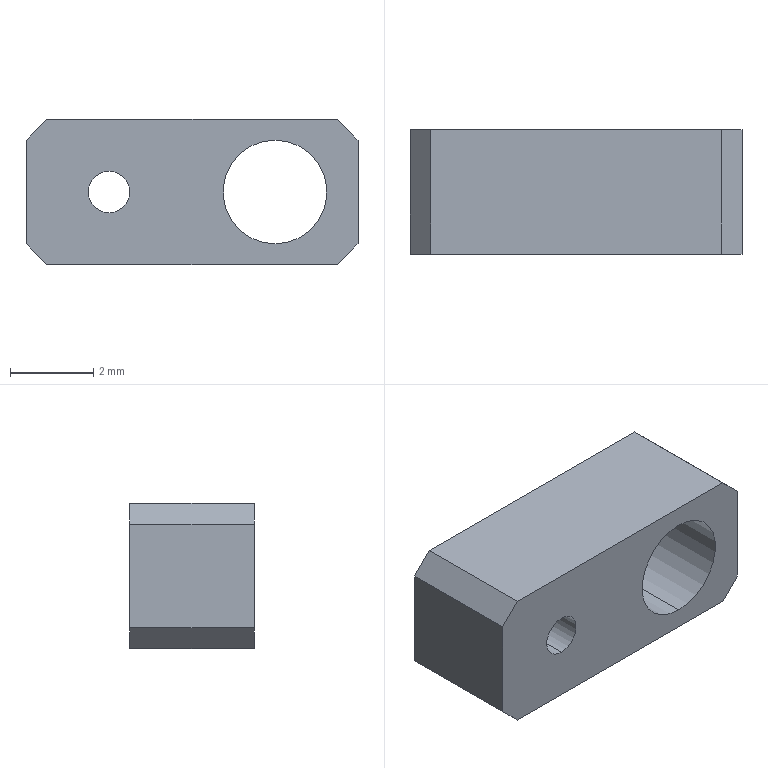Part | SolidWorks | features HoleWzd 2, Chamfer 1, Extrusion 1, ICE 1 | 1 solid | 17 faces | box 8 x 3 x 3.5 mm | volume 57.171 mm3 | plane 11 | cylinder 6 | commonest cylinder face diameters 2.5 x4 1 x2
STEP:
#1=CARTESIAN_POINT('',(2.,1.5,1.25));
#2=VERTEX_POINT('',#1);
#3=CARTESIAN_POINT('',(2.,1.5,-1.25));
#4=VERTEX_POINT('',#3);
#5=CARTESIAN_POINT('',(2.,1.5,0.));
#6=DIRECTION('',(0.,-1.,0.));
#7=DIRECTION('',(0.,0.,-1.));
#8=AXIS2_PLACEMENT_3D('',#5,#6,#7);
#9=CIRCLE('',#8,1.25);
#10=EDGE_CURVE('',#2,#4,#9,.T.);
#11=ORIENTED_EDGE('',*,*,#10,.F.);
#12=CARTESIAN_POINT('',(2.,-1.5,1.25));
#13=VERTEX_POINT('',#12);
#14=CARTESIAN_POINT('',(2.,-1.5,1.25));
#15=DIRECTION('',(0.,-1.,0.));
#16=VECTOR('',#15,1000.);
#17=LINE('',#14,#16);
#18=EDGE_CURVE('',#2,#13,#17,.T.);
#19=ORIENTED_EDGE('',*,*,#18,.T.);
#20=CARTESIAN_POINT('',(2.,-1.5,-1.25));
#21=VERTEX_POINT('',#20);
#22=CARTESIAN_POINT('',(2.,-1.5,0.));
#23=DIRECTION('',(0.,-1.,0.));
#24=DIRECTION('',(0.,0.,-1.));
#25=AXIS2_PLACEMENT_3D('',#22,#23,#24);
#26=CIRCLE('',#25,1.25);
#27=EDGE_CURVE('',#13,#21,#26,.T.);
#28=ORIENTED_EDGE('',*,*,#27,.T.);
#29=CARTESIAN_POINT('',(2.,-1.5,-1.25));
#30=DIRECTION('',(0.,-1.,0.));
#31=VECTOR('',#30,1000.);
#32=LINE('',#29,#31);
#33=EDGE_CURVE('',#4,#21,#32,.T.);
#34=ORIENTED_EDGE('',*,*,#33,.F.);
#35=EDGE_LOOP('',(#11,#19,#28,#34));
#36=FACE_OUTER_BOUND('',#35,.T.);
#37=CARTESIAN_POINT('',(2.,-1.5,0.));
#38=DIRECTION('',(0.,-1.,0.));
#39=DIRECTION('',(0.,0.,-1.));
#40=AXIS2_PLACEMENT_3D('',#37,#38,#39);
#41=CYLINDRICAL_SURFACE('',#40,1.25);
#42=ADVANCED_FACE('',(#36),#41,.F.);
#43=CARTESIAN_POINT('',(-2.,-0.5,-0.5));
#44=VERTEX_POINT('',#43);
#45=CARTESIAN_POINT('',(-2.,-0.5,0.5));
#46=VERTEX_POINT('',#45);
#47=CARTESIAN_POINT('',(-2.,-0.5,0.));
#48=DIRECTION('',(0.,1.,0.));
#49=DIRECTION('',(0.,0.,1.));
#50=AXIS2_PLACEMENT_3D('',#47,#48,#49);
#51=CIRCLE('',#50,0.5);
#52=EDGE_CURVE('',#44,#46,#51,.T.);
#53=ORIENTED_EDGE('',*,*,#52,.T.);
#54=CARTESIAN_POINT('',(-2.,-1.5,0.5));
#55=VERTEX_POINT('',#54);
#56=CARTESIAN_POINT('',(-2.,-1.5,0.5));
#57=DIRECTION('',(0.,-1.,0.));
#58=VECTOR('',#57,1000.);
#59=LINE('',#56,#58);
#60=EDGE_CURVE('',#46,#55,#59,.T.);
#61=ORIENTED_EDGE('',*,*,#60,.T.);
#62=CARTESIAN_POINT('',(-2.,-1.5,-0.5));
#63=VERTEX_POINT('',#62);
#64=CARTESIAN_POINT('',(-2.,-1.5,0.));
#65=DIRECTION('',(0.,-1.,0.));
#66=DIRECTION('',(0.,0.,-1.));
#67=AXIS2_PLACEMENT_3D('',#64,#65,#66);
#68=CIRCLE('',#67,0.5);
#69=EDGE_CURVE('',#55,#63,#68,.T.);
#70=ORIENTED_EDGE('',*,*,#69,.T.);
#71=CARTESIAN_POINT('',(-2.,-1.5,-0.5));
#72=DIRECTION('',(0.,-1.,0.));
#73=VECTOR('',#72,1000.);
#74=LINE('',#71,#73);
#75=EDGE_CURVE('',#44,#63,#74,.T.);
#76=ORIENTED_EDGE('',*,*,#75,.F.);
#77=EDGE_LOOP('',(#53,#61,#70,#76));
#78=FACE_OUTER_BOUND('',#77,.T.);
#79=CARTESIAN_POINT('',(-2.,-1.5,0.));
#80=DIRECTION('',(0.,-1.,0.));
#81=DIRECTION('',(0.,0.,-1.));
#82=AXIS2_PLACEMENT_3D('',#79,#80,#81);
#83=CYLINDRICAL_SURFACE('',#82,0.5);
#84=ADVANCED_FACE('',(#78),#83,.F.);
#85=CARTESIAN_POINT('',(-2.,-0.5,-1.25));
#86=VERTEX_POINT('',#85);
#87=CARTESIAN_POINT('',(-2.,-0.5,1.25));
#88=VERTEX_POINT('',#87);
#89=CARTESIAN_POINT('',(-2.,-0.5,0.));
#90=DIRECTION('',(0.,1.,0.));
#91=DIRECTION('',(0.,0.,1.));
#92=AXIS2_PLACEMENT_3D('',#89,#90,#91);
#93=CIRCLE('',#92,1.25);
#94=EDGE_CURVE('',#86,#88,#93,.T.);
#95=ORIENTED_EDGE('',*,*,#94,.F.);
#96=CARTESIAN_POINT('',(-2.,1.5,-1.25));
#97=VERTEX_POINT('',#96);
#98=CARTESIAN_POINT('',(-2.,-0.5,-1.25));
#99=DIRECTION('',(0.,1.,0.));
#100=VECTOR('',#99,1000.);
#101=LINE('',#98,#100);
#102=EDGE_CURVE('',#86,#97,#101,.T.);
#103=ORIENTED_EDGE('',*,*,#102,.T.);
#104=CARTESIAN_POINT('',(-2.,1.5,1.25));
#105=VERTEX_POINT('',#104);
#106=CARTESIAN_POINT('',(-2.,1.5,0.));
#107=DIRECTION('',(0.,1.,0.));
#108=DIRECTION('',(0.,0.,1.));
#109=AXIS2_PLACEMENT_3D('',#106,#107,#108);
#110=CIRCLE('',#109,1.25);
#111=EDGE_CURVE('',#97,#105,#110,.T.);
#112=ORIENTED_EDGE('',*,*,#111,.T.);
#113=CARTESIAN_POINT('',(-2.,-0.5,1.25));
#114=DIRECTION('',(0.,1.,0.));
#115=VECTOR('',#114,1000.);
#116=LINE('',#113,#115);
#117=EDGE_CURVE('',#88,#105,#116,.T.);
#118=ORIENTED_EDGE('',*,*,#117,.F.);
#119=EDGE_LOOP('',(#95,#103,#112,#118));
#120=FACE_OUTER_BOUND('',#119,.T.);
#121=CARTESIAN_POINT('',(-2.,-0.5,0.));
#122=DIRECTION('',(0.,1.,0.));
#123=DIRECTION('',(0.,0.,1.));
#124=AXIS2_PLACEMENT_3D('',#121,#122,#123);
#125=CYLINDRICAL_SURFACE('',#124,1.25);
#126=ADVANCED_FACE('',(#120),#125,.F.);
#127=CARTESIAN_POINT('',(4.,1.5,1.25));
#128=VERTEX_POINT('',#127);
#129=CARTESIAN_POINT('',(4.,1.5,-1.25));
#130=VERTEX_POINT('',#129);
#131=CARTESIAN_POINT('',(4.,1.5,-1.75));
#132=DIRECTION('',(0.,0.,-1.));
#133=VECTOR('',#132,1000.);
#134=LINE('',#131,#133);
#135=EDGE_CURVE('',#128,#130,#134,.T.);
#136=ORIENTED_EDGE('',*,*,#135,.F.);
#137=CARTESIAN_POINT('',(4.,-1.5,1.25));
#138=VERTEX_POINT('',#137);
#139=CARTESIAN_POINT('',(4.,1.5,1.25));
#140=DIRECTION('',(0.,-1.,0.));
#141=VECTOR('',#140,1000.);
#142=LINE('',#139,#141);
#143=EDGE_CURVE('',#128,#138,#142,.T.);
#144=ORIENTED_EDGE('',*,*,#143,.T.);
#145=CARTESIAN_POINT('',(4.,-1.5,-1.25));
#146=VERTEX_POINT('',#145);
#147=CARTESIAN_POINT('',(4.,-1.5,-1.75));
#148=DIRECTION('',(0.,0.,-1.));
#149=VECTOR('',#148,1000.);
#150=LINE('',#147,#149);
#151=EDGE_CURVE('',#138,#146,#150,.T.);
#152=ORIENTED_EDGE('',*,*,#151,.T.);
#153=CARTESIAN_POINT('',(4.,1.5,-1.25));
#154=DIRECTION('',(0.,1.,0.));
#155=VECTOR('',#154,1000.);
#156=LINE('',#153,#155);
#157=EDGE_CURVE('',#146,#130,#156,.T.);
#158=ORIENTED_EDGE('',*,*,#157,.T.);
#159=EDGE_LOOP('',(#136,#144,#152,#158));
#160=FACE_OUTER_BOUND('',#159,.T.);
#161=CARTESIAN_POINT('',(4.,1.5,-1.75));
#162=DIRECTION('',(-1.,0.,0.));
#163=DIRECTION('',(0.,0.,1.));
#164=AXIS2_PLACEMENT_3D('',#161,#162,#163);
#165=PLANE('',#164);
#166=ADVANCED_FACE('',(#160),#165,.F.);
#167=CARTESIAN_POINT('',(3.5,1.5,-1.75));
#168=VERTEX_POINT('',#167);
#169=CARTESIAN_POINT('',(-3.5,1.5,-1.75));
#170=VERTEX_POINT('',#169);
#171=CARTESIAN_POINT('',(-4.,1.5,-1.75));
#172=DIRECTION('',(-1.,0.,0.));
#173=VECTOR('',#172,1000.);
#174=LINE('',#171,#173);
#175=EDGE_CURVE('',#168,#170,#174,.T.);
#176=ORIENTED_EDGE('',*,*,#175,.F.);
#177=CARTESIAN_POINT('',(3.5,-1.5,-1.75));
#178=VERTEX_POINT('',#177);
#179=CARTESIAN_POINT('',(3.5,1.5,-1.75));
#180=DIRECTION('',(0.,-1.,0.));
#181=VECTOR('',#180,1000.);
#182=LINE('',#179,#181);
#183=EDGE_CURVE('',#168,#178,#182,.T.);
#184=ORIENTED_EDGE('',*,*,#183,.T.);
#185=CARTESIAN_POINT('',(-3.5,-1.5,-1.75));
#186=VERTEX_POINT('',#185);
#187=CARTESIAN_POINT('',(-4.,-1.5,-1.75));
#188=DIRECTION('',(-1.,0.,0.));
#189=VECTOR('',#188,1000.);
#190=LINE('',#187,#189);
#191=EDGE_CURVE('',#178,#186,#190,.T.);
#192=ORIENTED_EDGE('',*,*,#191,.T.);
#193=CARTESIAN_POINT('',(-3.5,1.5,-1.75));
#194=DIRECTION('',(0.,1.,0.));
#195=VECTOR('',#194,1000.);
#196=LINE('',#193,#195);
#197=EDGE_CURVE('',#186,#170,#196,.T.);
#198=ORIENTED_EDGE('',*,*,#197,.T.);
#199=EDGE_LOOP('',(#176,#184,#192,#198));
#200=FACE_OUTER_BOUND('',#199,.T.);
#201=CARTESIAN_POINT('',(-4.,1.5,-1.75));
#202=DIRECTION('',(0.,0.,1.));
#203=DIRECTION('',(1.,0.,0.));
#204=AXIS2_PLACEMENT_3D('',#201,#202,#203);
#205=PLANE('',#204);
#206=ADVANCED_FACE('',(#200),#205,.F.);
#207=CARTESIAN_POINT('',(-4.,-1.5,-1.25));
#208=VERTEX_POINT('',#207);
#209=CARTESIAN_POINT('',(-4.,-1.5,1.25));
#210=VERTEX_POINT('',#209);
#211=CARTESIAN_POINT('',(-4.,-1.5,-1.75));
#212=DIRECTION('',(0.,0.,1.));
#213=VECTOR('',#212,1000.);
#214=LINE('',#211,#213);
#215=EDGE_CURVE('',#208,#210,#214,.T.);
#216=ORIENTED_EDGE('',*,*,#215,.T.);
#217=CARTESIAN_POINT('',(-4.,1.5,1.25));
#218=VERTEX_POINT('',#217);
#219=CARTESIAN_POINT('',(-4.,1.5,1.25));
#220=DIRECTION('',(0.,1.,0.));
#221=VECTOR('',#220,1000.);
#222=LINE('',#219,#221);
#223=EDGE_CURVE('',#210,#218,#222,.T.);
#224=ORIENTED_EDGE('',*,*,#223,.T.);
#225=CARTESIAN_POINT('',(-4.,1.5,-1.25));
#226=VERTEX_POINT('',#225);
#227=CARTESIAN_POINT('',(-4.,1.5,-1.75));
#228=DIRECTION('',(0.,0.,1.));
#229=VECTOR('',#228,1000.);
#230=LINE('',#227,#229);
#231=EDGE_CURVE('',#226,#218,#230,.T.);
#232=ORIENTED_EDGE('',*,*,#231,.F.);
#233=CARTESIAN_POINT('',(-4.,1.5,-1.25));
#234=DIRECTION('',(0.,-1.,0.));
#235=VECTOR('',#234,1000.);
#236=LINE('',#233,#235);
#237=EDGE_CURVE('',#226,#208,#236,.T.);
#238=ORIENTED_EDGE('',*,*,#237,.T.);
#239=EDGE_LOOP('',(#216,#224,#232,#238));
#240=FACE_OUTER_BOUND('',#239,.T.);
#241=CARTESIAN_POINT('',(-4.,1.5,-1.75));
#242=DIRECTION('',(1.,0.,0.));
#243=DIRECTION('',(0.,0.,-1.));
#244=AXIS2_PLACEMENT_3D('',#241,#242,#243);
#245=PLANE('',#244);
#246=ADVANCED_FACE('',(#240),#245,.F.);
#247=CARTESIAN_POINT('',(-3.5,-1.5,1.75));
#248=VERTEX_POINT('',#247);
#249=CARTESIAN_POINT('',(3.5,-1.5,1.75));
#250=VERTEX_POINT('',#249);
#251=CARTESIAN_POINT('',(-4.,-1.5,1.75));
#252=DIRECTION('',(1.,0.,0.));
#253=VECTOR('',#252,1000.);
#254=LINE('',#251,#253);
#255=EDGE_CURVE('',#248,#250,#254,.T.);
#256=ORIENTED_EDGE('',*,*,#255,.T.);
#257=CARTESIAN_POINT('',(3.5,1.5,1.75));
#258=VERTEX_POINT('',#257);
#259=CARTESIAN_POINT('',(3.5,1.5,1.75));
#260=DIRECTION('',(0.,1.,0.));
#261=VECTOR('',#260,1000.);
#262=LINE('',#259,#261);
#263=EDGE_CURVE('',#250,#258,#262,.T.);
#264=ORIENTED_EDGE('',*,*,#263,.T.);
#265=CARTESIAN_POINT('',(-3.5,1.5,1.75));
#266=VERTEX_POINT('',#265);
#267=CARTESIAN_POINT('',(-4.,1.5,1.75));
#268=DIRECTION('',(1.,0.,0.));
#269=VECTOR('',#268,1000.);
#270=LINE('',#267,#269);
#271=EDGE_CURVE('',#266,#258,#270,.T.);
#272=ORIENTED_EDGE('',*,*,#271,.F.);
#273=CARTESIAN_POINT('',(-3.5,1.5,1.75));
#274=DIRECTION('',(0.,-1.,0.));
#275=VECTOR('',#274,1000.);
#276=LINE('',#273,#275);
#277=EDGE_CURVE('',#266,#248,#276,.T.);
#278=ORIENTED_EDGE('',*,*,#277,.T.);
#279=EDGE_LOOP('',(#256,#264,#272,#278));
#280=FACE_OUTER_BOUND('',#279,.T.);
#281=CARTESIAN_POINT('',(-4.,1.5,1.75));
#282=DIRECTION('',(0.,0.,-1.));
#283=DIRECTION('',(-1.,0.,0.));
#284=AXIS2_PLACEMENT_3D('',#281,#282,#283);
#285=PLANE('',#284);
#286=ADVANCED_FACE('',(#280),#285,.F.);
#287=CARTESIAN_POINT('',(2.,1.5,0.));
#288=DIRECTION('',(0.,-1.,0.));
#289=DIRECTION('',(0.,0.,-1.));
#290=AXIS2_PLACEMENT_3D('',#287,#288,#289);
#291=CIRCLE('',#290,1.25);
#292=EDGE_CURVE('',#4,#2,#291,.T.);
#293=ORIENTED_EDGE('',*,*,#292,.T.);
#294=ORIENTED_EDGE('',*,*,#10,.T.);
#295=EDGE_LOOP('',(#293,#294));
#296=FACE_BOUND('',#295,.T.);
#297=CARTESIAN_POINT('',(-2.,1.5,0.));
#298=DIRECTION('',(0.,1.,0.));
#299=DIRECTION('',(0.,0.,1.));
#300=AXIS2_PLACEMENT_3D('',#297,#298,#299);
#301=CIRCLE('',#300,1.25);
#302=EDGE_CURVE('',#105,#97,#301,.T.);
#303=ORIENTED_EDGE('',*,*,#302,.F.);
#304=ORIENTED_EDGE('',*,*,#111,.F.);
#305=EDGE_LOOP('',(#303,#304));
#306=FACE_BOUND('',#305,.T.);
#307=ORIENTED_EDGE('',*,*,#271,.T.);
#308=CARTESIAN_POINT('',(2.625,1.5,2.625));
#309=DIRECTION('',(0.7071,0.,-0.7071));
#310=VECTOR('',#309,1000.);
#311=LINE('',#308,#310);
#312=EDGE_CURVE('',#258,#128,#311,.T.);
#313=ORIENTED_EDGE('',*,*,#312,.T.);
#314=ORIENTED_EDGE('',*,*,#135,.T.);
#315=CARTESIAN_POINT('',(2.625,1.5,-2.625));
#316=DIRECTION('',(-0.7071,0.,-0.7071));
#317=VECTOR('',#316,1000.);
#318=LINE('',#315,#317);
#319=EDGE_CURVE('',#130,#168,#318,.T.);
#320=ORIENTED_EDGE('',*,*,#319,.T.);
#321=ORIENTED_EDGE('',*,*,#175,.T.);
#322=CARTESIAN_POINT('',(-2.625,1.5,-2.625));
#323=DIRECTION('',(-0.7071,0.,0.7071));
#324=VECTOR('',#323,1000.);
#325=LINE('',#322,#324);
#326=EDGE_CURVE('',#170,#226,#325,.T.);
#327=ORIENTED_EDGE('',*,*,#326,.T.);
#328=ORIENTED_EDGE('',*,*,#231,.T.);
#329=CARTESIAN_POINT('',(-2.625,1.5,2.625));
#330=DIRECTION('',(0.7071,0.,0.7071));
#331=VECTOR('',#330,1000.);
#332=LINE('',#329,#331);
#333=EDGE_CURVE('',#218,#266,#332,.T.);
#334=ORIENTED_EDGE('',*,*,#333,.T.);
#335=EDGE_LOOP('',(#307,#313,#314,#320,#321,#327,#328,#334));
#336=FACE_OUTER_BOUND('',#335,.T.);
#337=CARTESIAN_POINT('',(0.,1.5,0.));
#338=DIRECTION('',(0.,1.,0.));
#339=DIRECTION('',(0.,0.,1.));
#340=AXIS2_PLACEMENT_3D('',#337,#338,#339);
#341=PLANE('',#340);
#342=ADVANCED_FACE('',(#296,#306,#336),#341,.T.);
#343=CARTESIAN_POINT('',(2.,-1.5,0.));
#344=DIRECTION('',(0.,-1.,0.));
#345=DIRECTION('',(0.,0.,-1.));
#346=AXIS2_PLACEMENT_3D('',#343,#344,#345);
#347=CIRCLE('',#346,1.25);
#348=EDGE_CURVE('',#21,#13,#347,.T.);
#349=ORIENTED_EDGE('',*,*,#348,.F.);
#350=ORIENTED_EDGE('',*,*,#27,.F.);
#351=EDGE_LOOP('',(#349,#350));
#352=FACE_BOUND('',#351,.T.);
#353=CARTESIAN_POINT('',(-2.,-1.5,0.));
#354=DIRECTION('',(0.,-1.,0.));
#355=DIRECTION('',(0.,0.,-1.));
#356=AXIS2_PLACEMENT_3D('',#353,#354,#355);
#357=CIRCLE('',#356,0.5);
#358=EDGE_CURVE('',#63,#55,#357,.T.);
#359=ORIENTED_EDGE('',*,*,#358,.F.);
#360=ORIENTED_EDGE('',*,*,#69,.F.);
#361=EDGE_LOOP('',(#359,#360));
#362=FACE_BOUND('',#361,.T.);
#363=ORIENTED_EDGE('',*,*,#151,.F.);
#364=CARTESIAN_POINT('',(4.,-1.5,1.25));
#365=DIRECTION('',(-0.7071,0.,0.7071));
#366=VECTOR('',#365,1000.);
#367=LINE('',#364,#366);
#368=EDGE_CURVE('',#138,#250,#367,.T.);
#369=ORIENTED_EDGE('',*,*,#368,.T.);
#370=ORIENTED_EDGE('',*,*,#255,.F.);
#371=CARTESIAN_POINT('',(-3.5,-1.5,1.75));
#372=DIRECTION('',(-0.7071,0.,-0.7071));
#373=VECTOR('',#372,1000.);
#374=LINE('',#371,#373);
#375=EDGE_CURVE('',#248,#210,#374,.T.);
#376=ORIENTED_EDGE('',*,*,#375,.T.);
#377=ORIENTED_EDGE('',*,*,#215,.F.);
#378=CARTESIAN_POINT('',(-4.,-1.5,-1.25));
#379=DIRECTION('',(0.7071,0.,-0.7071));
#380=VECTOR('',#379,1000.);
#381=LINE('',#378,#380);
#382=EDGE_CURVE('',#208,#186,#381,.T.);
#383=ORIENTED_EDGE('',*,*,#382,.T.);
#384=ORIENTED_EDGE('',*,*,#191,.F.);
#385=CARTESIAN_POINT('',(3.5,-1.5,-1.75));
#386=DIRECTION('',(0.7071,0.,0.7071));
#387=VECTOR('',#386,1000.);
#388=LINE('',#385,#387);
#389=EDGE_CURVE('',#178,#146,#388,.T.);
#390=ORIENTED_EDGE('',*,*,#389,.T.);
#391=EDGE_LOOP('',(#363,#369,#370,#376,#377,#383,#384,#390));
#392=FACE_OUTER_BOUND('',#391,.T.);
#393=CARTESIAN_POINT('',(0.,-1.5,0.));
#394=DIRECTION('',(0.,1.,0.));
#395=DIRECTION('',(0.,0.,1.));
#396=AXIS2_PLACEMENT_3D('',#393,#394,#395);
#397=PLANE('',#396);
#398=ADVANCED_FACE('',(#352,#362,#392),#397,.F.);
#399=ORIENTED_EDGE('',*,*,#102,.F.);
#400=CARTESIAN_POINT('',(-2.,-0.5,0.));
#401=DIRECTION('',(0.,1.,0.));
#402=DIRECTION('',(0.,0.,1.));
#403=AXIS2_PLACEMENT_3D('',#400,#401,#402);
#404=CIRCLE('',#403,1.25);
#405=EDGE_CURVE('',#88,#86,#404,.T.);
#406=ORIENTED_EDGE('',*,*,#405,.F.);
#407=ORIENTED_EDGE('',*,*,#117,.T.);
#408=ORIENTED_EDGE('',*,*,#302,.T.);
#409=EDGE_LOOP('',(#399,#406,#407,#408));
#410=FACE_OUTER_BOUND('',#409,.T.);
#411=CARTESIAN_POINT('',(-2.,-0.5,0.));
#412=DIRECTION('',(0.,1.,0.));
#413=DIRECTION('',(0.,0.,1.));
#414=AXIS2_PLACEMENT_3D('',#411,#412,#413);
#415=CYLINDRICAL_SURFACE('',#414,1.25);
#416=ADVANCED_FACE('',(#410),#415,.F.);
#417=ORIENTED_EDGE('',*,*,#52,.F.);
#418=CARTESIAN_POINT('',(-2.,-0.5,0.));
#419=DIRECTION('',(0.,1.,0.));
#420=DIRECTION('',(0.,0.,1.));
#421=AXIS2_PLACEMENT_3D('',#418,#419,#420);
#422=CIRCLE('',#421,0.5);
#423=EDGE_CURVE('',#46,#44,#422,.T.);
#424=ORIENTED_EDGE('',*,*,#423,.F.);
#425=EDGE_LOOP('',(#417,#424));
#426=FACE_BOUND('',#425,.T.);
#427=ORIENTED_EDGE('',*,*,#405,.T.);
#428=ORIENTED_EDGE('',*,*,#94,.T.);
#429=EDGE_LOOP('',(#427,#428));
#430=FACE_OUTER_BOUND('',#429,.T.);
#431=CARTESIAN_POINT('',(-2.,-0.5,0.));
#432=DIRECTION('',(0.,1.,0.));
#433=DIRECTION('',(0.,0.,1.));
#434=AXIS2_PLACEMENT_3D('',#431,#432,#433);
#435=PLANE('',#434);
#436=ADVANCED_FACE('',(#426,#430),#435,.T.);
#437=ORIENTED_EDGE('',*,*,#312,.F.);
#438=ORIENTED_EDGE('',*,*,#263,.F.);
#439=ORIENTED_EDGE('',*,*,#368,.F.);
#440=ORIENTED_EDGE('',*,*,#143,.F.);
#441=EDGE_LOOP('',(#437,#438,#439,#440));
#442=FACE_OUTER_BOUND('',#441,.T.);
#443=CARTESIAN_POINT('',(4.,1.5,1.25));
#444=DIRECTION('',(-0.7071,0.,-0.7071));
#445=DIRECTION('',(0.,-1.,0.));
#446=AXIS2_PLACEMENT_3D('',#443,#444,#445);
#447=PLANE('',#446);
#448=ADVANCED_FACE('',(#442),#447,.F.);
#449=ORIENTED_EDGE('',*,*,#319,.F.);
#450=ORIENTED_EDGE('',*,*,#157,.F.);
#451=ORIENTED_EDGE('',*,*,#389,.F.);
#452=ORIENTED_EDGE('',*,*,#183,.F.);
#453=EDGE_LOOP('',(#449,#450,#451,#452));
#454=FACE_OUTER_BOUND('',#453,.T.);
#455=CARTESIAN_POINT('',(3.5,1.5,-1.75));
#456=DIRECTION('',(-0.7071,0.,0.7071));
#457=DIRECTION('',(0.,-1.,0.));
#458=AXIS2_PLACEMENT_3D('',#455,#456,#457);
#459=PLANE('',#458);
#460=ADVANCED_FACE('',(#454),#459,.F.);
#461=ORIENTED_EDGE('',*,*,#333,.F.);
#462=ORIENTED_EDGE('',*,*,#223,.F.);
#463=ORIENTED_EDGE('',*,*,#375,.F.);
#464=ORIENTED_EDGE('',*,*,#277,.F.);
#465=EDGE_LOOP('',(#461,#462,#463,#464));
#466=FACE_OUTER_BOUND('',#465,.T.);
#467=CARTESIAN_POINT('',(-3.5,1.5,1.75));
#468=DIRECTION('',(0.7071,0.,-0.7071));
#469=DIRECTION('',(0.,-1.,0.));
#470=AXIS2_PLACEMENT_3D('',#467,#468,#469);
#471=PLANE('',#470);
#472=ADVANCED_FACE('',(#466),#471,.F.);
#473=ORIENTED_EDGE('',*,*,#326,.F.);
#474=ORIENTED_EDGE('',*,*,#197,.F.);
#475=ORIENTED_EDGE('',*,*,#382,.F.);
#476=ORIENTED_EDGE('',*,*,#237,.F.);
#477=EDGE_LOOP('',(#473,#474,#475,#476));
#478=FACE_OUTER_BOUND('',#477,.T.);
#479=CARTESIAN_POINT('',(-4.,1.5,-1.25));
#480=DIRECTION('',(0.7071,0.,0.7071));
#481=DIRECTION('',(0.,-1.,0.));
#482=AXIS2_PLACEMENT_3D('',#479,#480,#481);
#483=PLANE('',#482);
#484=ADVANCED_FACE('',(#478),#483,.F.);
#485=ORIENTED_EDGE('',*,*,#60,.F.);
#486=ORIENTED_EDGE('',*,*,#423,.T.);
#487=ORIENTED_EDGE('',*,*,#75,.T.);
#488=ORIENTED_EDGE('',*,*,#358,.T.);
#489=EDGE_LOOP('',(#485,#486,#487,#488));
#490=FACE_OUTER_BOUND('',#489,.T.);
#491=CARTESIAN_POINT('',(-2.,-1.5,0.));
#492=DIRECTION('',(0.,-1.,0.));
#493=DIRECTION('',(0.,0.,-1.));
#494=AXIS2_PLACEMENT_3D('',#491,#492,#493);
#495=CYLINDRICAL_SURFACE('',#494,0.5);
#496=ADVANCED_FACE('',(#490),#495,.F.);
#497=ORIENTED_EDGE('',*,*,#18,.F.);
#498=ORIENTED_EDGE('',*,*,#292,.F.);
#499=ORIENTED_EDGE('',*,*,#33,.T.);
#500=ORIENTED_EDGE('',*,*,#348,.T.);
#501=EDGE_LOOP('',(#497,#498,#499,#500));
#502=FACE_OUTER_BOUND('',#501,.T.);
#503=CARTESIAN_POINT('',(2.,-1.5,0.));
#504=DIRECTION('',(0.,-1.,0.));
#505=DIRECTION('',(0.,0.,-1.));
#506=AXIS2_PLACEMENT_3D('',#503,#504,#505);
#507=CYLINDRICAL_SURFACE('',#506,1.25);
#508=ADVANCED_FACE('',(#502),#507,.F.);
#509=CLOSED_SHELL('',(#42,#84,#126,#166,#206,#246,#286,#342,#398,#416,#436,#448,#460,#472,#484,#496,#508));
#510=MANIFOLD_SOLID_BREP('',#509);
#511=CARTESIAN_POINT('',(0.,0.,0.));
#512=DIRECTION('',(0.,0.,1.));
#513=DIRECTION('',(1.,0.,0.));
#514=AXIS2_PLACEMENT_3D('',#511,#512,#513);
#515=(LENGTH_UNIT()NAMED_UNIT(*)SI_UNIT(.MILLI.,.METRE.));
#516=UNCERTAINTY_MEASURE_WITH_UNIT(LENGTH_MEASURE(0.00001),#515,'','');
#517=(NAMED_UNIT(*)PLANE_ANGLE_UNIT()SI_UNIT($,.RADIAN.));
#518=(NAMED_UNIT(*)SI_UNIT($,.STERADIAN.)SOLID_ANGLE_UNIT());
#519=(GEOMETRIC_REPRESENTATION_CONTEXT(3)GLOBAL_UNCERTAINTY_ASSIGNED_CONTEXT((#516))GLOBAL_UNIT_ASSIGNED_CONTEXT((#515,#517,#518))REPRESENTATION_CONTEXT('',''));
#520=ADVANCED_BREP_SHAPE_REPRESENTATION('',(#510,#514),#519);